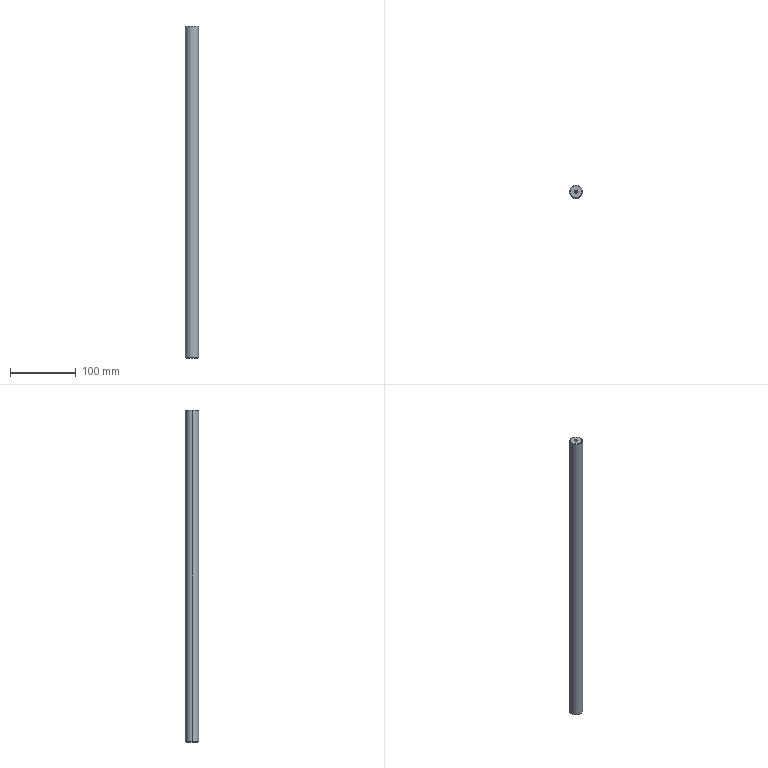Part | STEP file | Guide rod | 1 solid | 12 faces | box 20 x 20 x 505 mm | volume 158440 mm3 | cone 6 | cylinder 4 | plane 2 | commonest cylinder face diameters 4.2 x2 20 x2
STEP:
#1=CARTESIAN_POINT('',(0.,0.,0.));
#2=DIRECTION('',(0.,0.,1.));
#3=DIRECTION('',(1.,0.,0.));
#4=AXIS2_PLACEMENT_3D('',#1,#2,#3);
#5=CARTESIAN_POINT('',(2.1,0.,494.6));
#6=VERTEX_POINT('',#5);
#7=CARTESIAN_POINT('',(2.1,0.,505.));
#8=VERTEX_POINT('',#7);
#9=CARTESIAN_POINT('',(2.1,0.,505.));
#10=DIRECTION('',(0.,0.,1.));
#11=VECTOR('',#10,1.);
#12=LINE('',#9,#11);
#13=CARTESIAN_POINT('',(0.,0.,505.));
#14=DIRECTION('',(0.,0.,1.));
#15=DIRECTION('',(1.,0.,0.));
#16=AXIS2_PLACEMENT_3D('',#13,#14,#15);
#17=CYLINDRICAL_SURFACE('',#16,2.1);
#18=CARTESIAN_POINT('',(6.283,0.));
#19=DIRECTION('',(0.,1.));
#20=VECTOR('',#19,1.);
#21=LINE('',#18,#20);
#22=(GEOMETRIC_REPRESENTATION_CONTEXT(2)PARAMETRIC_REPRESENTATION_CONTEXT()REPRESENTATION_CONTEXT('',''));
#23=DEFINITIONAL_REPRESENTATION('',(#21),#22);
#24=PCURVE('',#17,#23);
#25=CARTESIAN_POINT('',(0.,0.,505.));
#26=DIRECTION('',(0.,0.,1.));
#27=DIRECTION('',(1.,0.,0.));
#28=AXIS2_PLACEMENT_3D('',#25,#26,#27);
#29=CYLINDRICAL_SURFACE('',#28,2.1);
#30=CARTESIAN_POINT('',(0.,0.));
#31=DIRECTION('',(0.,1.));
#32=VECTOR('',#31,1.);
#33=LINE('',#30,#32);
#34=(GEOMETRIC_REPRESENTATION_CONTEXT(2)PARAMETRIC_REPRESENTATION_CONTEXT()REPRESENTATION_CONTEXT('',''));
#35=DEFINITIONAL_REPRESENTATION('',(#33),#34);
#36=PCURVE('',#29,#35);
#37=SURFACE_CURVE('',#12,(#24,#36),.PCURVE_S1.);
#38=EDGE_CURVE('',#6,#8,#37,.T.);
#39=ORIENTED_EDGE('',*,*,#38,.T.);
#40=CARTESIAN_POINT('',(-2.1,0.,505.));
#41=VERTEX_POINT('',#40);
#42=CARTESIAN_POINT('',(0.,0.,505.));
#43=DIRECTION('',(0.,0.,1.));
#44=DIRECTION('',(1.,0.,0.));
#45=AXIS2_PLACEMENT_3D('',#42,#43,#44);
#46=CIRCLE('',#45,2.1);
#47=CARTESIAN_POINT('',(0.,0.));
#48=DIRECTION('',(1.,0.));
#49=VECTOR('',#48,1.);
#50=LINE('',#47,#49);
#51=(GEOMETRIC_REPRESENTATION_CONTEXT(2)PARAMETRIC_REPRESENTATION_CONTEXT()REPRESENTATION_CONTEXT('',''));
#52=DEFINITIONAL_REPRESENTATION('',(#50),#51);
#53=PCURVE('',#17,#52);
#54=CARTESIAN_POINT('',(0.,0.,505.));
#55=DIRECTION('',(0.,0.,1.));
#56=DIRECTION('',(1.,0.,0.));
#57=AXIS2_PLACEMENT_3D('',#54,#55,#56);
#58=PLANE('',#57);
#59=CARTESIAN_POINT('',(0.,0.));
#60=DIRECTION('',(1.,0.));
#61=AXIS2_PLACEMENT_2D('',#59,#60);
#62=CIRCLE('',#61,2.1);
#63=(GEOMETRIC_REPRESENTATION_CONTEXT(2)PARAMETRIC_REPRESENTATION_CONTEXT()REPRESENTATION_CONTEXT('',''));
#64=DEFINITIONAL_REPRESENTATION('',(#62),#63);
#65=PCURVE('',#58,#64);
#66=SURFACE_CURVE('',#46,(#53,#65),.PCURVE_S1.);
#67=EDGE_CURVE('',#41,#8,#66,.T.);
#68=ORIENTED_EDGE('',*,*,#67,.F.);
#69=CARTESIAN_POINT('',(-2.1,0.,494.6));
#70=VERTEX_POINT('',#69);
#71=CARTESIAN_POINT('',(-2.1,0.,505.));
#72=DIRECTION('',(0.,0.,1.));
#73=VECTOR('',#72,1.);
#74=LINE('',#71,#73);
#75=CARTESIAN_POINT('',(3.142,0.));
#76=DIRECTION('',(0.,1.));
#77=VECTOR('',#76,1.);
#78=LINE('',#75,#77);
#79=(GEOMETRIC_REPRESENTATION_CONTEXT(2)PARAMETRIC_REPRESENTATION_CONTEXT()REPRESENTATION_CONTEXT('',''));
#80=DEFINITIONAL_REPRESENTATION('',(#78),#79);
#81=PCURVE('',#17,#80);
#82=CARTESIAN_POINT('',(3.142,0.));
#83=DIRECTION('',(0.,1.));
#84=VECTOR('',#83,1.);
#85=LINE('',#82,#84);
#86=(GEOMETRIC_REPRESENTATION_CONTEXT(2)PARAMETRIC_REPRESENTATION_CONTEXT()REPRESENTATION_CONTEXT('',''));
#87=DEFINITIONAL_REPRESENTATION('',(#85),#86);
#88=PCURVE('',#29,#87);
#89=SURFACE_CURVE('',#74,(#81,#88),.PCURVE_S1.);
#90=EDGE_CURVE('',#70,#41,#89,.T.);
#91=ORIENTED_EDGE('',*,*,#90,.F.);
#92=CARTESIAN_POINT('',(0.,0.,494.6));
#93=DIRECTION('',(0.,0.,1.));
#94=DIRECTION('',(1.,0.,0.));
#95=AXIS2_PLACEMENT_3D('',#92,#93,#94);
#96=CIRCLE('',#95,2.1);
#97=CARTESIAN_POINT('',(0.,-10.4));
#98=DIRECTION('',(1.,0.));
#99=VECTOR('',#98,1.);
#100=LINE('',#97,#99);
#101=(GEOMETRIC_REPRESENTATION_CONTEXT(2)PARAMETRIC_REPRESENTATION_CONTEXT()REPRESENTATION_CONTEXT('',''));
#102=DEFINITIONAL_REPRESENTATION('',(#100),#101);
#103=PCURVE('',#17,#102);
#104=CARTESIAN_POINT('',(0.,0.,494.6));
#105=DIRECTION('',(0.,0.,1.));
#106=DIRECTION('',(1.,0.,0.));
#107=AXIS2_PLACEMENT_3D('',#104,#105,#106);
#108=CONICAL_SURFACE('',#107,2.1,1.03);
#109=CARTESIAN_POINT('',(0.,0.));
#110=DIRECTION('',(1.,0.));
#111=VECTOR('',#110,1.);
#112=LINE('',#109,#111);
#113=(GEOMETRIC_REPRESENTATION_CONTEXT(2)PARAMETRIC_REPRESENTATION_CONTEXT()REPRESENTATION_CONTEXT('',''));
#114=DEFINITIONAL_REPRESENTATION('',(#112),#113);
#115=PCURVE('',#108,#114);
#116=SURFACE_CURVE('',#96,(#103,#115),.PCURVE_S1.);
#117=EDGE_CURVE('',#70,#6,#116,.T.);
#118=ORIENTED_EDGE('',*,*,#117,.T.);
#119=EDGE_LOOP('',(#39,#68,#91,#118));
#120=FACE_BOUND('',#119,.F.);
#121=ADVANCED_FACE('',(#120),#17,.F.);
#122=ORIENTED_EDGE('',*,*,#117,.F.);
#123=CARTESIAN_POINT('',(0.,0.,493.338));
#124=VERTEX_POINT('',#123);
#125=CARTESIAN_POINT('',(-2.1,0.,494.6));
#126=DIRECTION('',(-0.8572,0.,0.515));
#127=VECTOR('',#126,1.);
#128=LINE('',#125,#127);
#129=CARTESIAN_POINT('',(3.142,0.));
#130=DIRECTION('',(0.,1.));
#131=VECTOR('',#130,1.);
#132=LINE('',#129,#131);
#133=(GEOMETRIC_REPRESENTATION_CONTEXT(2)PARAMETRIC_REPRESENTATION_CONTEXT()REPRESENTATION_CONTEXT('',''));
#134=DEFINITIONAL_REPRESENTATION('',(#132),#133);
#135=PCURVE('',#108,#134);
#136=CARTESIAN_POINT('',(0.,0.,494.6));
#137=DIRECTION('',(0.,0.,1.));
#138=DIRECTION('',(1.,0.,0.));
#139=AXIS2_PLACEMENT_3D('',#136,#137,#138);
#140=CONICAL_SURFACE('',#139,2.1,1.03);
#141=CARTESIAN_POINT('',(3.142,0.));
#142=DIRECTION('',(0.,1.));
#143=VECTOR('',#142,1.);
#144=LINE('',#141,#143);
#145=(GEOMETRIC_REPRESENTATION_CONTEXT(2)PARAMETRIC_REPRESENTATION_CONTEXT()REPRESENTATION_CONTEXT('',''));
#146=DEFINITIONAL_REPRESENTATION('',(#144),#145);
#147=PCURVE('',#140,#146);
#148=SURFACE_CURVE('',#128,(#135,#147),.PCURVE_S1.);
#149=EDGE_CURVE('',#124,#70,#148,.T.);
#150=ORIENTED_EDGE('',*,*,#149,.F.);
#151=CARTESIAN_POINT('',(2.1,0.,494.6));
#152=DIRECTION('',(0.8572,0.,0.515));
#153=VECTOR('',#152,1.);
#154=LINE('',#151,#153);
#155=CARTESIAN_POINT('',(6.283,0.));
#156=DIRECTION('',(0.,1.));
#157=VECTOR('',#156,1.);
#158=LINE('',#155,#157);
#159=(GEOMETRIC_REPRESENTATION_CONTEXT(2)PARAMETRIC_REPRESENTATION_CONTEXT()REPRESENTATION_CONTEXT('',''));
#160=DEFINITIONAL_REPRESENTATION('',(#158),#159);
#161=PCURVE('',#108,#160);
#162=CARTESIAN_POINT('',(0.,0.));
#163=DIRECTION('',(0.,1.));
#164=VECTOR('',#163,1.);
#165=LINE('',#162,#164);
#166=(GEOMETRIC_REPRESENTATION_CONTEXT(2)PARAMETRIC_REPRESENTATION_CONTEXT()REPRESENTATION_CONTEXT('',''));
#167=DEFINITIONAL_REPRESENTATION('',(#165),#166);
#168=PCURVE('',#140,#167);
#169=SURFACE_CURVE('',#154,(#161,#168),.PCURVE_S1.);
#170=EDGE_CURVE('',#124,#6,#169,.T.);
#171=ORIENTED_EDGE('',*,*,#170,.T.);
#172=EDGE_LOOP('',(#122,#150,#171));
#173=FACE_BOUND('',#172,.F.);
#174=ADVANCED_FACE('',(#173),#108,.F.);
#175=CARTESIAN_POINT('',(9.,0.,505.));
#176=VERTEX_POINT('',#175);
#177=CARTESIAN_POINT('',(-9.,0.,505.));
#178=VERTEX_POINT('',#177);
#179=CARTESIAN_POINT('',(0.,0.,505.));
#180=DIRECTION('',(0.,0.,1.));
#181=DIRECTION('',(1.,0.,0.));
#182=AXIS2_PLACEMENT_3D('',#179,#180,#181);
#183=CIRCLE('',#182,9.);
#184=CARTESIAN_POINT('',(0.,0.,505.));
#185=DIRECTION('',(0.,0.,-1.));
#186=DIRECTION('',(-1.,0.,0.));
#187=AXIS2_PLACEMENT_3D('',#184,#185,#186);
#188=CONICAL_SURFACE('',#187,9.,0.7854);
#189=CARTESIAN_POINT('',(3.142,0.));
#190=DIRECTION('',(-1.,0.));
#191=VECTOR('',#190,1.);
#192=LINE('',#189,#191);
#193=(GEOMETRIC_REPRESENTATION_CONTEXT(2)PARAMETRIC_REPRESENTATION_CONTEXT()REPRESENTATION_CONTEXT('',''));
#194=DEFINITIONAL_REPRESENTATION('',(#192),#193);
#195=PCURVE('',#188,#194);
#196=CARTESIAN_POINT('',(0.,0.));
#197=DIRECTION('',(1.,0.));
#198=AXIS2_PLACEMENT_2D('',#196,#197);
#199=CIRCLE('',#198,9.);
#200=(GEOMETRIC_REPRESENTATION_CONTEXT(2)PARAMETRIC_REPRESENTATION_CONTEXT()REPRESENTATION_CONTEXT('',''));
#201=DEFINITIONAL_REPRESENTATION('',(#199),#200);
#202=PCURVE('',#58,#201);
#203=SURFACE_CURVE('',#183,(#195,#202),.PCURVE_S1.);
#204=EDGE_CURVE('',#176,#178,#203,.T.);
#205=ORIENTED_EDGE('',*,*,#204,.F.);
#206=CARTESIAN_POINT('',(10.,0.,504.));
#207=VERTEX_POINT('',#206);
#208=CARTESIAN_POINT('',(9.,0.,505.));
#209=DIRECTION('',(0.7071,0.,-0.7071));
#210=VECTOR('',#209,1.);
#211=LINE('',#208,#210);
#212=CARTESIAN_POINT('',(3.142,0.));
#213=DIRECTION('',(0.,1.));
#214=VECTOR('',#213,1.);
#215=LINE('',#212,#214);
#216=(GEOMETRIC_REPRESENTATION_CONTEXT(2)PARAMETRIC_REPRESENTATION_CONTEXT()REPRESENTATION_CONTEXT('',''));
#217=DEFINITIONAL_REPRESENTATION('',(#215),#216);
#218=PCURVE('',#188,#217);
#219=CARTESIAN_POINT('',(0.,0.,505.));
#220=DIRECTION('',(0.,0.,-1.));
#221=DIRECTION('',(-1.,0.,0.));
#222=AXIS2_PLACEMENT_3D('',#219,#220,#221);
#223=CONICAL_SURFACE('',#222,9.,0.7854);
#224=CARTESIAN_POINT('',(3.142,0.));
#225=DIRECTION('',(0.,1.));
#226=VECTOR('',#225,1.);
#227=LINE('',#224,#226);
#228=(GEOMETRIC_REPRESENTATION_CONTEXT(2)PARAMETRIC_REPRESENTATION_CONTEXT()REPRESENTATION_CONTEXT('',''));
#229=DEFINITIONAL_REPRESENTATION('',(#227),#228);
#230=PCURVE('',#223,#229);
#231=SURFACE_CURVE('',#211,(#218,#230),.PCURVE_S1.);
#232=EDGE_CURVE('',#176,#207,#231,.T.);
#233=ORIENTED_EDGE('',*,*,#232,.T.);
#234=CARTESIAN_POINT('',(-10.,0.,504.));
#235=VERTEX_POINT('',#234);
#236=CARTESIAN_POINT('',(0.,0.,504.));
#237=DIRECTION('',(0.,0.,-1.));
#238=DIRECTION('',(1.,0.,0.));
#239=AXIS2_PLACEMENT_3D('',#236,#237,#238);
#240=CIRCLE('',#239,10.);
#241=CARTESIAN_POINT('',(-3.142,1.));
#242=DIRECTION('',(1.,0.));
#243=VECTOR('',#242,1.);
#244=LINE('',#241,#243);
#245=(GEOMETRIC_REPRESENTATION_CONTEXT(2)PARAMETRIC_REPRESENTATION_CONTEXT()REPRESENTATION_CONTEXT('',''));
#246=DEFINITIONAL_REPRESENTATION('',(#244),#245);
#247=PCURVE('',#188,#246);
#248=CARTESIAN_POINT('',(0.,0.,505.));
#249=DIRECTION('',(0.,0.,-1.));
#250=DIRECTION('',(-1.,0.,0.));
#251=AXIS2_PLACEMENT_3D('',#248,#249,#250);
#252=CYLINDRICAL_SURFACE('',#251,10.);
#253=CARTESIAN_POINT('',(-3.142,1.));
#254=DIRECTION('',(1.,0.));
#255=VECTOR('',#254,1.);
#256=LINE('',#253,#255);
#257=(GEOMETRIC_REPRESENTATION_CONTEXT(2)PARAMETRIC_REPRESENTATION_CONTEXT()REPRESENTATION_CONTEXT('',''));
#258=DEFINITIONAL_REPRESENTATION('',(#256),#257);
#259=PCURVE('',#252,#258);
#260=SURFACE_CURVE('',#240,(#247,#259),.PCURVE_S1.);
#261=EDGE_CURVE('',#235,#207,#260,.T.);
#262=ORIENTED_EDGE('',*,*,#261,.F.);
#263=CARTESIAN_POINT('',(-9.,0.,505.));
#264=DIRECTION('',(-0.7071,0.,-0.7071));
#265=VECTOR('',#264,1.);
#266=LINE('',#263,#265);
#267=CARTESIAN_POINT('',(0.,0.));
#268=DIRECTION('',(0.,1.));
#269=VECTOR('',#268,1.);
#270=LINE('',#267,#269);
#271=(GEOMETRIC_REPRESENTATION_CONTEXT(2)PARAMETRIC_REPRESENTATION_CONTEXT()REPRESENTATION_CONTEXT('',''));
#272=DEFINITIONAL_REPRESENTATION('',(#270),#271);
#273=PCURVE('',#188,#272);
#274=CARTESIAN_POINT('',(6.283,0.));
#275=DIRECTION('',(0.,1.));
#276=VECTOR('',#275,1.);
#277=LINE('',#274,#276);
#278=(GEOMETRIC_REPRESENTATION_CONTEXT(2)PARAMETRIC_REPRESENTATION_CONTEXT()REPRESENTATION_CONTEXT('',''));
#279=DEFINITIONAL_REPRESENTATION('',(#277),#278);
#280=PCURVE('',#223,#279);
#281=SURFACE_CURVE('',#266,(#273,#280),.PCURVE_S1.);
#282=EDGE_CURVE('',#178,#235,#281,.T.);
#283=ORIENTED_EDGE('',*,*,#282,.F.);
#284=EDGE_LOOP('',(#205,#233,#262,#283));
#285=FACE_BOUND('',#284,.T.);
#286=ADVANCED_FACE('',(#285),#188,.T.);
#287=CARTESIAN_POINT('',(-9.,0.,0.));
#288=VERTEX_POINT('',#287);
#289=CARTESIAN_POINT('',(9.,0.,0.));
#290=VERTEX_POINT('',#289);
#291=CARTESIAN_POINT('',(0.,0.,0.));
#292=DIRECTION('',(0.,0.,-1.));
#293=DIRECTION('',(1.,0.,0.));
#294=AXIS2_PLACEMENT_3D('',#291,#292,#293);
#295=CIRCLE('',#294,9.);
#296=CARTESIAN_POINT('',(0.,0.,1.));
#297=DIRECTION('',(0.,0.,1.));
#298=DIRECTION('',(1.,0.,0.));
#299=AXIS2_PLACEMENT_3D('',#296,#297,#298);
#300=CONICAL_SURFACE('',#299,10.,0.7854);
#301=CARTESIAN_POINT('',(6.283,-1.));
#302=DIRECTION('',(-1.,0.));
#303=VECTOR('',#302,1.);
#304=LINE('',#301,#303);
#305=(GEOMETRIC_REPRESENTATION_CONTEXT(2)PARAMETRIC_REPRESENTATION_CONTEXT()REPRESENTATION_CONTEXT('',''));
#306=DEFINITIONAL_REPRESENTATION('',(#304),#305);
#307=PCURVE('',#300,#306);
#308=CARTESIAN_POINT('',(0.,0.,0.));
#309=DIRECTION('',(0.,0.,1.));
#310=DIRECTION('',(1.,0.,0.));
#311=AXIS2_PLACEMENT_3D('',#308,#309,#310);
#312=PLANE('',#311);
#313=CARTESIAN_POINT('',(9.,0.));
#314=CARTESIAN_POINT('',(9.,-15.588));
#315=CARTESIAN_POINT('',(-4.5,-7.794));
#316=CARTESIAN_POINT('',(-18.,0.));
#317=CARTESIAN_POINT('',(-4.5,7.794));
#318=CARTESIAN_POINT('',(9.,15.588));
#319=CARTESIAN_POINT('',(9.,0.));
#320=(BOUNDED_CURVE()B_SPLINE_CURVE(2,(#313,#314,#315,#316,#317,#318,#319),.UNSPECIFIED.,.T.,.F.)B_SPLINE_CURVE_WITH_KNOTS((1,2,2,2,2,1),(-2.094,0.,2.094,4.189,6.283,8.378),.UNSPECIFIED.)CURVE()GEOMETRIC_REPRESENTATION_ITEM()RATIONAL_B_SPLINE_CURVE((1.,0.5,1.,0.5,1.,0.5,1.))REPRESENTATION_ITEM(''));
#321=(GEOMETRIC_REPRESENTATION_CONTEXT(2)PARAMETRIC_REPRESENTATION_CONTEXT()REPRESENTATION_CONTEXT('',''));
#322=DEFINITIONAL_REPRESENTATION('',(#320),#321);
#323=PCURVE('',#312,#322);
#324=SURFACE_CURVE('',#295,(#307,#323),.PCURVE_S1.);
#325=EDGE_CURVE('',#288,#290,#324,.T.);
#326=ORIENTED_EDGE('',*,*,#325,.F.);
#327=CARTESIAN_POINT('',(-10.,0.,1.));
#328=VERTEX_POINT('',#327);
#329=CARTESIAN_POINT('',(-10.,0.,1.));
#330=DIRECTION('',(-0.7071,0.,0.7071));
#331=VECTOR('',#330,1.);
#332=LINE('',#329,#331);
#333=CARTESIAN_POINT('',(3.142,0.));
#334=DIRECTION('',(0.,1.));
#335=VECTOR('',#334,1.);
#336=LINE('',#333,#335);
#337=(GEOMETRIC_REPRESENTATION_CONTEXT(2)PARAMETRIC_REPRESENTATION_CONTEXT()REPRESENTATION_CONTEXT('',''));
#338=DEFINITIONAL_REPRESENTATION('',(#336),#337);
#339=PCURVE('',#300,#338);
#340=CARTESIAN_POINT('',(0.,0.,1.));
#341=DIRECTION('',(0.,0.,1.));
#342=DIRECTION('',(1.,0.,0.));
#343=AXIS2_PLACEMENT_3D('',#340,#341,#342);
#344=CONICAL_SURFACE('',#343,10.,0.7854);
#345=CARTESIAN_POINT('',(3.142,0.));
#346=DIRECTION('',(0.,1.));
#347=VECTOR('',#346,1.);
#348=LINE('',#345,#347);
#349=(GEOMETRIC_REPRESENTATION_CONTEXT(2)PARAMETRIC_REPRESENTATION_CONTEXT()REPRESENTATION_CONTEXT('',''));
#350=DEFINITIONAL_REPRESENTATION('',(#348),#349);
#351=PCURVE('',#344,#350);
#352=SURFACE_CURVE('',#332,(#339,#351),.PCURVE_S1.);
#353=EDGE_CURVE('',#288,#328,#352,.T.);
#354=ORIENTED_EDGE('',*,*,#353,.T.);
#355=CARTESIAN_POINT('',(10.,0.,1.));
#356=VERTEX_POINT('',#355);
#357=CARTESIAN_POINT('',(0.,0.,1.));
#358=DIRECTION('',(0.,0.,1.));
#359=DIRECTION('',(1.,0.,0.));
#360=AXIS2_PLACEMENT_3D('',#357,#358,#359);
#361=CIRCLE('',#360,10.);
#362=CARTESIAN_POINT('',(0.,0.));
#363=DIRECTION('',(1.,0.));
#364=VECTOR('',#363,1.);
#365=LINE('',#362,#364);
#366=(GEOMETRIC_REPRESENTATION_CONTEXT(2)PARAMETRIC_REPRESENTATION_CONTEXT()REPRESENTATION_CONTEXT('',''));
#367=DEFINITIONAL_REPRESENTATION('',(#365),#366);
#368=PCURVE('',#300,#367);
#369=CARTESIAN_POINT('',(3.142,504.));
#370=DIRECTION('',(-1.,0.));
#371=VECTOR('',#370,1.);
#372=LINE('',#369,#371);
#373=(GEOMETRIC_REPRESENTATION_CONTEXT(2)PARAMETRIC_REPRESENTATION_CONTEXT()REPRESENTATION_CONTEXT('',''));
#374=DEFINITIONAL_REPRESENTATION('',(#372),#373);
#375=PCURVE('',#252,#374);
#376=SURFACE_CURVE('',#361,(#368,#375),.PCURVE_S1.);
#377=EDGE_CURVE('',#356,#328,#376,.T.);
#378=ORIENTED_EDGE('',*,*,#377,.F.);
#379=CARTESIAN_POINT('',(10.,0.,1.));
#380=DIRECTION('',(0.7071,0.,0.7071));
#381=VECTOR('',#380,1.);
#382=LINE('',#379,#381);
#383=CARTESIAN_POINT('',(0.,0.));
#384=DIRECTION('',(0.,1.));
#385=VECTOR('',#384,1.);
#386=LINE('',#383,#385);
#387=(GEOMETRIC_REPRESENTATION_CONTEXT(2)PARAMETRIC_REPRESENTATION_CONTEXT()REPRESENTATION_CONTEXT('',''));
#388=DEFINITIONAL_REPRESENTATION('',(#386),#387);
#389=PCURVE('',#300,#388);
#390=CARTESIAN_POINT('',(6.283,0.));
#391=DIRECTION('',(0.,1.));
#392=VECTOR('',#391,1.);
#393=LINE('',#390,#392);
#394=(GEOMETRIC_REPRESENTATION_CONTEXT(2)PARAMETRIC_REPRESENTATION_CONTEXT()REPRESENTATION_CONTEXT('',''));
#395=DEFINITIONAL_REPRESENTATION('',(#393),#394);
#396=PCURVE('',#344,#395);
#397=SURFACE_CURVE('',#382,(#389,#396),.PCURVE_S1.);
#398=EDGE_CURVE('',#290,#356,#397,.T.);
#399=ORIENTED_EDGE('',*,*,#398,.F.);
#400=EDGE_LOOP('',(#326,#354,#378,#399));
#401=FACE_BOUND('',#400,.T.);
#402=ADVANCED_FACE('',(#401),#300,.T.);
#403=ORIENTED_EDGE('',*,*,#261,.T.);
#404=CARTESIAN_POINT('',(10.,0.,505.));
#405=DIRECTION('',(0.,0.,-1.));
#406=VECTOR('',#405,1.);
#407=LINE('',#404,#406);
#408=CARTESIAN_POINT('',(3.142,0.));
#409=DIRECTION('',(0.,1.));
#410=VECTOR('',#409,1.);
#411=LINE('',#408,#410);
#412=(GEOMETRIC_REPRESENTATION_CONTEXT(2)PARAMETRIC_REPRESENTATION_CONTEXT()REPRESENTATION_CONTEXT('',''));
#413=DEFINITIONAL_REPRESENTATION('',(#411),#412);
#414=PCURVE('',#252,#413);
#415=CARTESIAN_POINT('',(0.,0.,505.));
#416=DIRECTION('',(0.,0.,-1.));
#417=DIRECTION('',(-1.,0.,0.));
#418=AXIS2_PLACEMENT_3D('',#415,#416,#417);
#419=CYLINDRICAL_SURFACE('',#418,10.);
#420=CARTESIAN_POINT('',(3.142,0.));
#421=DIRECTION('',(0.,1.));
#422=VECTOR('',#421,1.);
#423=LINE('',#420,#422);
#424=(GEOMETRIC_REPRESENTATION_CONTEXT(2)PARAMETRIC_REPRESENTATION_CONTEXT()REPRESENTATION_CONTEXT('',''));
#425=DEFINITIONAL_REPRESENTATION('',(#423),#424);
#426=PCURVE('',#419,#425);
#427=SURFACE_CURVE('',#407,(#414,#426),.PCURVE_S1.);
#428=EDGE_CURVE('',#207,#356,#427,.T.);
#429=ORIENTED_EDGE('',*,*,#428,.T.);
#430=ORIENTED_EDGE('',*,*,#377,.T.);
#431=CARTESIAN_POINT('',(-10.,0.,505.));
#432=DIRECTION('',(0.,0.,-1.));
#433=VECTOR('',#432,1.);
#434=LINE('',#431,#433);
#435=CARTESIAN_POINT('',(0.,0.));
#436=DIRECTION('',(0.,1.));
#437=VECTOR('',#436,1.);
#438=LINE('',#435,#437);
#439=(GEOMETRIC_REPRESENTATION_CONTEXT(2)PARAMETRIC_REPRESENTATION_CONTEXT()REPRESENTATION_CONTEXT('',''));
#440=DEFINITIONAL_REPRESENTATION('',(#438),#439);
#441=PCURVE('',#252,#440);
#442=CARTESIAN_POINT('',(6.283,0.));
#443=DIRECTION('',(0.,1.));
#444=VECTOR('',#443,1.);
#445=LINE('',#442,#444);
#446=(GEOMETRIC_REPRESENTATION_CONTEXT(2)PARAMETRIC_REPRESENTATION_CONTEXT()REPRESENTATION_CONTEXT('',''));
#447=DEFINITIONAL_REPRESENTATION('',(#445),#446);
#448=PCURVE('',#419,#447);
#449=SURFACE_CURVE('',#434,(#441,#448),.PCURVE_S1.);
#450=EDGE_CURVE('',#235,#328,#449,.T.);
#451=ORIENTED_EDGE('',*,*,#450,.F.);
#452=EDGE_LOOP('',(#403,#429,#430,#451));
#453=FACE_BOUND('',#452,.T.);
#454=ADVANCED_FACE('',(#453),#252,.T.);
#455=ORIENTED_EDGE('',*,*,#428,.F.);
#456=CARTESIAN_POINT('',(0.,0.,504.));
#457=DIRECTION('',(0.,0.,-1.));
#458=DIRECTION('',(1.,0.,0.));
#459=AXIS2_PLACEMENT_3D('',#456,#457,#458);
#460=CIRCLE('',#459,10.);
#461=CARTESIAN_POINT('',(3.142,1.));
#462=DIRECTION('',(1.,0.));
#463=VECTOR('',#462,1.);
#464=LINE('',#461,#463);
#465=(GEOMETRIC_REPRESENTATION_CONTEXT(2)PARAMETRIC_REPRESENTATION_CONTEXT()REPRESENTATION_CONTEXT('',''));
#466=DEFINITIONAL_REPRESENTATION('',(#464),#465);
#467=PCURVE('',#419,#466);
#468=CARTESIAN_POINT('',(3.142,1.));
#469=DIRECTION('',(1.,0.));
#470=VECTOR('',#469,1.);
#471=LINE('',#468,#470);
#472=(GEOMETRIC_REPRESENTATION_CONTEXT(2)PARAMETRIC_REPRESENTATION_CONTEXT()REPRESENTATION_CONTEXT('',''));
#473=DEFINITIONAL_REPRESENTATION('',(#471),#472);
#474=PCURVE('',#223,#473);
#475=SURFACE_CURVE('',#460,(#467,#474),.PCURVE_S1.);
#476=EDGE_CURVE('',#207,#235,#475,.T.);
#477=ORIENTED_EDGE('',*,*,#476,.T.);
#478=ORIENTED_EDGE('',*,*,#450,.T.);
#479=CARTESIAN_POINT('',(0.,0.,1.));
#480=DIRECTION('',(0.,0.,1.));
#481=DIRECTION('',(1.,0.,0.));
#482=AXIS2_PLACEMENT_3D('',#479,#480,#481);
#483=CIRCLE('',#482,10.);
#484=CARTESIAN_POINT('',(9.425,504.));
#485=DIRECTION('',(-1.,0.));
#486=VECTOR('',#485,1.);
#487=LINE('',#484,#486);
#488=(GEOMETRIC_REPRESENTATION_CONTEXT(2)PARAMETRIC_REPRESENTATION_CONTEXT()REPRESENTATION_CONTEXT('',''));
#489=DEFINITIONAL_REPRESENTATION('',(#487),#488);
#490=PCURVE('',#419,#489);
#491=CARTESIAN_POINT('',(0.,0.));
#492=DIRECTION('',(1.,0.));
#493=VECTOR('',#492,1.);
#494=LINE('',#491,#493);
#495=(GEOMETRIC_REPRESENTATION_CONTEXT(2)PARAMETRIC_REPRESENTATION_CONTEXT()REPRESENTATION_CONTEXT('',''));
#496=DEFINITIONAL_REPRESENTATION('',(#494),#495);
#497=PCURVE('',#344,#496);
#498=SURFACE_CURVE('',#483,(#490,#497),.PCURVE_S1.);
#499=EDGE_CURVE('',#328,#356,#498,.T.);
#500=ORIENTED_EDGE('',*,*,#499,.T.);
#501=EDGE_LOOP('',(#455,#477,#478,#500));
#502=FACE_BOUND('',#501,.T.);
#503=ADVANCED_FACE('',(#502),#419,.T.);
#504=CARTESIAN_POINT('',(0.,0.,505.));
#505=DIRECTION('',(0.,0.,1.));
#506=DIRECTION('',(1.,0.,0.));
#507=AXIS2_PLACEMENT_3D('',#504,#505,#506);
#508=CIRCLE('',#507,2.1);
#509=CARTESIAN_POINT('',(0.,0.));
#510=DIRECTION('',(1.,0.));
#511=AXIS2_PLACEMENT_2D('',#509,#510);
#512=CIRCLE('',#511,2.1);
#513=(GEOMETRIC_REPRESENTATION_CONTEXT(2)PARAMETRIC_REPRESENTATION_CONTEXT()REPRESENTATION_CONTEXT('',''));
#514=DEFINITIONAL_REPRESENTATION('',(#512),#513);
#515=PCURVE('',#58,#514);
#516=CARTESIAN_POINT('',(0.,0.));
#517=DIRECTION('',(1.,0.));
#518=VECTOR('',#517,1.);
#519=LINE('',#516,#518);
#520=(GEOMETRIC_REPRESENTATION_CONTEXT(2)PARAMETRIC_REPRESENTATION_CONTEXT()REPRESENTATION_CONTEXT('',''));
#521=DEFINITIONAL_REPRESENTATION('',(#519),#520);
#522=PCURVE('',#29,#521);
#523=SURFACE_CURVE('',#508,(#515,#522),.PCURVE_S1.);
#524=EDGE_CURVE('',#8,#41,#523,.T.);
#525=ORIENTED_EDGE('',*,*,#524,.F.);
#526=ORIENTED_EDGE('',*,*,#67,.F.);
#527=EDGE_LOOP('',(#525,#526));
#528=FACE_BOUND('',#527,.T.);
#529=CARTESIAN_POINT('',(0.,0.,505.));
#530=DIRECTION('',(0.,0.,1.));
#531=DIRECTION('',(1.,0.,0.));
#532=AXIS2_PLACEMENT_3D('',#529,#530,#531);
#533=CIRCLE('',#532,9.);
#534=CARTESIAN_POINT('',(0.,0.));
#535=DIRECTION('',(1.,0.));
#536=AXIS2_PLACEMENT_2D('',#534,#535);
#537=CIRCLE('',#536,9.);
#538=(GEOMETRIC_REPRESENTATION_CONTEXT(2)PARAMETRIC_REPRESENTATION_CONTEXT()REPRESENTATION_CONTEXT('',''));
#539=DEFINITIONAL_REPRESENTATION('',(#537),#538);
#540=PCURVE('',#58,#539);
#541=CARTESIAN_POINT('',(9.425,0.));
#542=DIRECTION('',(-1.,0.));
#543=VECTOR('',#542,1.);
#544=LINE('',#541,#543);
#545=(GEOMETRIC_REPRESENTATION_CONTEXT(2)PARAMETRIC_REPRESENTATION_CONTEXT()REPRESENTATION_CONTEXT('',''));
#546=DEFINITIONAL_REPRESENTATION('',(#544),#545);
#547=PCURVE('',#223,#546);
#548=SURFACE_CURVE('',#533,(#540,#547),.PCURVE_S1.);
#549=EDGE_CURVE('',#178,#176,#548,.T.);
#550=ORIENTED_EDGE('',*,*,#549,.T.);
#551=ORIENTED_EDGE('',*,*,#204,.T.);
#552=EDGE_LOOP('',(#550,#551));
#553=FACE_BOUND('',#552,.T.);
#554=ADVANCED_FACE('',(#528,#553),#58,.T.);
#555=CARTESIAN_POINT('',(0.,0.,0.));
#556=DIRECTION('',(0.,0.,-1.));
#557=DIRECTION('',(1.,0.,0.));
#558=AXIS2_PLACEMENT_3D('',#555,#556,#557);
#559=CIRCLE('',#558,9.);
#560=CARTESIAN_POINT('',(9.,0.));
#561=CARTESIAN_POINT('',(9.,-15.588));
#562=CARTESIAN_POINT('',(-4.5,-7.794));
#563=CARTESIAN_POINT('',(-18.,0.));
#564=CARTESIAN_POINT('',(-4.5,7.794));
#565=CARTESIAN_POINT('',(9.,15.588));
#566=CARTESIAN_POINT('',(9.,0.));
#567=(BOUNDED_CURVE()B_SPLINE_CURVE(2,(#560,#561,#562,#563,#564,#565,#566),.UNSPECIFIED.,.T.,.F.)B_SPLINE_CURVE_WITH_KNOTS((1,2,2,2,2,1),(-2.094,0.,2.094,4.189,6.283,8.378),.UNSPECIFIED.)CURVE()GEOMETRIC_REPRESENTATION_ITEM()RATIONAL_B_SPLINE_CURVE((1.,0.5,1.,0.5,1.,0.5,1.))REPRESENTATION_ITEM(''));
#568=(GEOMETRIC_REPRESENTATION_CONTEXT(2)PARAMETRIC_REPRESENTATION_CONTEXT()REPRESENTATION_CONTEXT('',''));
#569=DEFINITIONAL_REPRESENTATION('',(#567),#568);
#570=PCURVE('',#312,#569);
#571=CARTESIAN_POINT('',(6.283,-1.));
#572=DIRECTION('',(-1.,0.));
#573=VECTOR('',#572,1.);
#574=LINE('',#571,#573);
#575=(GEOMETRIC_REPRESENTATION_CONTEXT(2)PARAMETRIC_REPRESENTATION_CONTEXT()REPRESENTATION_CONTEXT('',''));
#576=DEFINITIONAL_REPRESENTATION('',(#574),#575);
#577=PCURVE('',#344,#576);
#578=SURFACE_CURVE('',#559,(#570,#577),.PCURVE_S1.);
#579=EDGE_CURVE('',#290,#288,#578,.T.);
#580=ORIENTED_EDGE('',*,*,#579,.T.);
#581=ORIENTED_EDGE('',*,*,#325,.T.);
#582=EDGE_LOOP('',(#580,#581));
#583=FACE_BOUND('',#582,.T.);
#584=ADVANCED_FACE('',(#583),#312,.F.);
#585=ORIENTED_EDGE('',*,*,#353,.F.);
#586=ORIENTED_EDGE('',*,*,#579,.F.);
#587=ORIENTED_EDGE('',*,*,#398,.T.);
#588=ORIENTED_EDGE('',*,*,#499,.F.);
#589=EDGE_LOOP('',(#585,#586,#587,#588));
#590=FACE_BOUND('',#589,.T.);
#591=ADVANCED_FACE('',(#590),#344,.T.);
#592=ORIENTED_EDGE('',*,*,#232,.F.);
#593=ORIENTED_EDGE('',*,*,#549,.F.);
#594=ORIENTED_EDGE('',*,*,#282,.T.);
#595=ORIENTED_EDGE('',*,*,#476,.F.);
#596=EDGE_LOOP('',(#592,#593,#594,#595));
#597=FACE_BOUND('',#596,.T.);
#598=ADVANCED_FACE('',(#597),#223,.T.);
#599=CARTESIAN_POINT('',(0.,0.,494.6));
#600=DIRECTION('',(0.,0.,1.));
#601=DIRECTION('',(1.,0.,0.));
#602=AXIS2_PLACEMENT_3D('',#599,#600,#601);
#603=CIRCLE('',#602,2.1);
#604=CARTESIAN_POINT('',(0.,0.));
#605=DIRECTION('',(1.,0.));
#606=VECTOR('',#605,1.);
#607=LINE('',#604,#606);
#608=(GEOMETRIC_REPRESENTATION_CONTEXT(2)PARAMETRIC_REPRESENTATION_CONTEXT()REPRESENTATION_CONTEXT('',''));
#609=DEFINITIONAL_REPRESENTATION('',(#607),#608);
#610=PCURVE('',#140,#609);
#611=CARTESIAN_POINT('',(0.,-10.4));
#612=DIRECTION('',(1.,0.));
#613=VECTOR('',#612,1.);
#614=LINE('',#611,#613);
#615=(GEOMETRIC_REPRESENTATION_CONTEXT(2)PARAMETRIC_REPRESENTATION_CONTEXT()REPRESENTATION_CONTEXT('',''));
#616=DEFINITIONAL_REPRESENTATION('',(#614),#615);
#617=PCURVE('',#29,#616);
#618=SURFACE_CURVE('',#603,(#610,#617),.PCURVE_S1.);
#619=EDGE_CURVE('',#6,#70,#618,.T.);
#620=ORIENTED_EDGE('',*,*,#619,.F.);
#621=ORIENTED_EDGE('',*,*,#170,.F.);
#622=ORIENTED_EDGE('',*,*,#149,.T.);
#623=EDGE_LOOP('',(#620,#621,#622));
#624=FACE_BOUND('',#623,.F.);
#625=ADVANCED_FACE('',(#624),#140,.F.);
#626=ORIENTED_EDGE('',*,*,#524,.F.);
#627=ORIENTED_EDGE('',*,*,#38,.F.);
#628=ORIENTED_EDGE('',*,*,#619,.T.);
#629=ORIENTED_EDGE('',*,*,#90,.T.);
#630=EDGE_LOOP('',(#626,#627,#628,#629));
#631=FACE_BOUND('',#630,.F.);
#632=ADVANCED_FACE('',(#631),#29,.F.);
#633=CLOSED_SHELL('',(#121,#174,#286,#402,#454,#503,#554,#584,#591,#598,#625,#632));
#634=MANIFOLD_SOLID_BREP('',#633);
#635=(LENGTH_UNIT()NAMED_UNIT(*)SI_UNIT(.MILLI.,.METRE.));
#636=UNCERTAINTY_MEASURE_WITH_UNIT(LENGTH_MEASURE(0.0000001),#635,'','');
#637=(NAMED_UNIT(*)PLANE_ANGLE_UNIT()SI_UNIT($,.RADIAN.));
#638=(NAMED_UNIT(*)SI_UNIT($,.STERADIAN.)SOLID_ANGLE_UNIT());
#639=(GEOMETRIC_REPRESENTATION_CONTEXT(3)GLOBAL_UNCERTAINTY_ASSIGNED_CONTEXT((#636))GLOBAL_UNIT_ASSIGNED_CONTEXT((#635,#637,#638))REPRESENTATION_CONTEXT('',''));
#640=ADVANCED_BREP_SHAPE_REPRESENTATION('',(#4,#634),#639);